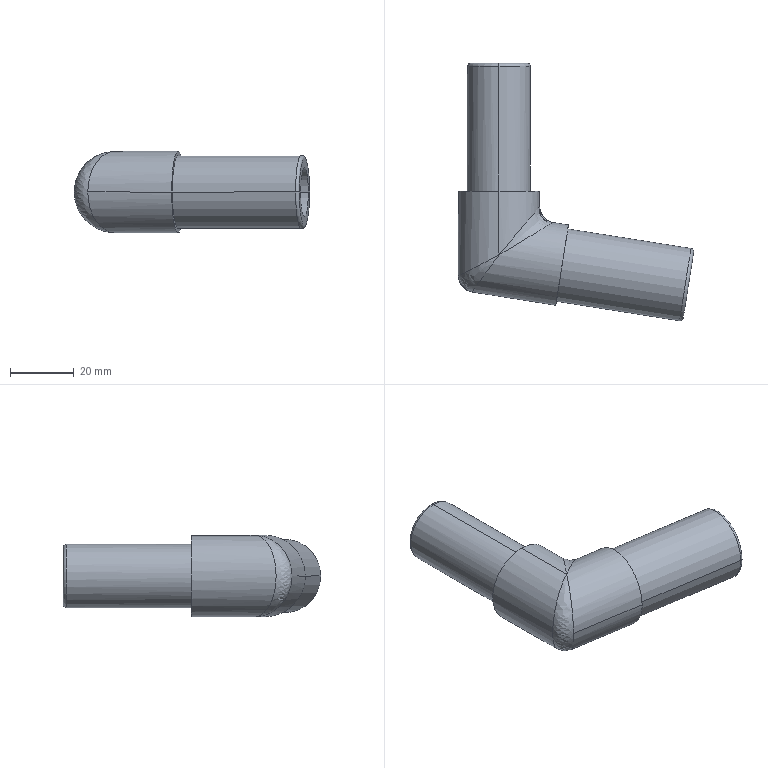Part | STEP file | 101000007608 | 1 solid | 25 faces | box 73.608 x 80.551 x 25.4 mm | volume 31663 mm3 | cylinder 14 | plane 5 | torus 4 | spline 2 | commonest cylinder face diameters 12.5 x4 25.4 x4 15.5 x2 19.8 x2 22.9 x2
STEP:
#1=CARTESIAN_POINT('',(-1.446,-20.539,0.));
#2=VERTEX_POINT('',#1);
#3=CARTESIAN_POINT('',(2.136,2.079,0.));
#4=VERTEX_POINT('',#3);
#5=CARTESIAN_POINT('',(0.345,-9.23,0.));
#6=DIRECTION('',(0.9877,-0.1564,0.));
#7=AXIS2_PLACEMENT_3D('',#5,#6,$);
#8=CIRCLE('',#7,11.45);
#9=EDGE_CURVE('',#2,#4,#8,.F.);
#10=ORIENTED_EDGE('',*,*,#9,.F.);
#11=CARTESIAN_POINT('',(-0.302,-19.707,0.));
#12=VERTEX_POINT('',#11);
#13=CARTESIAN_POINT('',(-1.29,-19.551,0.));
#14=DIRECTION('',(0.,0.,1.));
#15=AXIS2_PLACEMENT_3D('',#13,#14,$);
#16=CIRCLE('',#15,1.);
#17=EDGE_CURVE('',#2,#12,#16,.T.);
#18=ORIENTED_EDGE('',*,*,#17,.T.);
#19=CARTESIAN_POINT('',(2.967,0.9353,0.));
#20=VERTEX_POINT('',#19);
#21=CARTESIAN_POINT('',(1.333,-9.386,0.));
#22=DIRECTION('',(0.9877,-0.1564,0.));
#23=AXIS2_PLACEMENT_3D('',#21,#22,$);
#24=CIRCLE('',#23,10.45);
#25=EDGE_CURVE('',#20,#12,#24,.T.);
#26=ORIENTED_EDGE('',*,*,#25,.F.);
#27=CARTESIAN_POINT('',(1.98,1.092,0.));
#28=DIRECTION('',(0.,0.,-1.));
#29=AXIS2_PLACEMENT_3D('',#27,#28,$);
#30=CIRCLE('',#29,1.);
#31=EDGE_CURVE('',#4,#20,#30,.T.);
#32=ORIENTED_EDGE('',*,*,#31,.F.);
#33=EDGE_LOOP('',(#10,#18,#26,#32));
#34=FACE_OUTER_BOUND('',#33,.T.);
#35=CARTESIAN_POINT('',(0.345,-9.23,0.));
#36=DIRECTION('',(0.9877,-0.1564,0.));
#37=DIRECTION('',(0.1564,0.9877,0.));
#38=AXIS2_PLACEMENT_3D('',#35,#36,#37);
#39=TOROIDAL_SURFACE('',#38,10.45,1.);
#40=ADVANCED_FACE('',(#34),#39,.T.);
#41=ORIENTED_EDGE('',*,*,#9,.T.);
#42=CARTESIAN_POINT('',(-36.384,8.18,0.));
#43=VERTEX_POINT('',#42);
#44=CARTESIAN_POINT('',(3.124,1.923,0.));
#45=DIRECTION('',(-0.9877,0.1564,0.));
#46=VECTOR('',#45,1.);
#47=LINE('',#44,#46);
#48=EDGE_CURVE('',#4,#43,#47,.T.);
#49=ORIENTED_EDGE('',*,*,#48,.T.);
#50=CARTESIAN_POINT('',(-39.966,-14.438,0.));
#51=VERTEX_POINT('',#50);
#52=CARTESIAN_POINT('',(-38.175,-3.129,0.));
#53=DIRECTION('',(-0.9877,0.1564,0.));
#54=AXIS2_PLACEMENT_3D('',#52,#53,$);
#55=CIRCLE('',#54,11.45);
#56=EDGE_CURVE('',#43,#51,#55,.F.);
#57=ORIENTED_EDGE('',*,*,#56,.T.);
#58=CARTESIAN_POINT('',(-0.4585,-20.695,0.));
#59=DIRECTION('',(-0.9877,0.1564,0.));
#60=VECTOR('',#59,1.);
#61=LINE('',#58,#60);
#62=EDGE_CURVE('',#2,#51,#61,.T.);
#63=ORIENTED_EDGE('',*,*,#62,.F.);
#64=EDGE_LOOP('',(#41,#49,#57,#63));
#65=FACE_OUTER_BOUND('',#64,.T.);
#66=CARTESIAN_POINT('',(1.333,-9.386,0.));
#67=DIRECTION('',(-0.9877,0.1564,0.));
#68=DIRECTION('',(-0.1564,-0.9877,0.));
#69=AXIS2_PLACEMENT_3D('',#66,#67,#68);
#70=CYLINDRICAL_SURFACE('',#69,11.45);
#71=ADVANCED_FACE('',(#65),#70,.T.);
#72=ORIENTED_EDGE('',*,*,#17,.F.);
#73=CARTESIAN_POINT('',(0.345,-9.23,0.));
#74=DIRECTION('',(0.9877,-0.1564,0.));
#75=AXIS2_PLACEMENT_3D('',#73,#74,$);
#76=CIRCLE('',#75,11.45);
#77=EDGE_CURVE('',#4,#2,#76,.F.);
#78=ORIENTED_EDGE('',*,*,#77,.F.);
#79=ORIENTED_EDGE('',*,*,#31,.T.);
#80=CARTESIAN_POINT('',(1.333,-9.386,0.));
#81=DIRECTION('',(0.9877,-0.1564,0.));
#82=AXIS2_PLACEMENT_3D('',#80,#81,$);
#83=CIRCLE('',#82,10.45);
#84=EDGE_CURVE('',#12,#20,#83,.T.);
#85=ORIENTED_EDGE('',*,*,#84,.F.);
#86=EDGE_LOOP('',(#72,#78,#79,#85));
#87=FACE_OUTER_BOUND('',#86,.T.);
#88=CARTESIAN_POINT('',(0.345,-9.23,0.));
#89=DIRECTION('',(0.9877,-0.1564,0.));
#90=DIRECTION('',(-0.1564,-0.9877,0.));
#91=AXIS2_PLACEMENT_3D('',#88,#89,#90);
#92=TOROIDAL_SURFACE('',#91,10.45,1.);
#93=ADVANCED_FACE('',(#87),#92,.T.);
#94=ORIENTED_EDGE('',*,*,#25,.T.);
#95=ORIENTED_EDGE('',*,*,#84,.T.);
#96=EDGE_LOOP('',(#94,#95));
#97=FACE_OUTER_BOUND('',#96,.T.);
#98=CARTESIAN_POINT('',(2.545,-1.731,0.));
#99=VERTEX_POINT('',#98);
#100=CARTESIAN_POINT('',(0.1204,-17.041,0.));
#101=VERTEX_POINT('',#100);
#102=CARTESIAN_POINT('',(1.333,-9.386,0.));
#103=DIRECTION('',(0.9877,-0.1564,0.));
#104=AXIS2_PLACEMENT_3D('',#102,#103,$);
#105=CIRCLE('',#104,7.75);
#106=EDGE_CURVE('',#99,#101,#105,.T.);
#107=ORIENTED_EDGE('',*,*,#106,.F.);
#108=CARTESIAN_POINT('',(1.333,-9.386,0.));
#109=DIRECTION('',(0.9877,-0.1564,0.));
#110=AXIS2_PLACEMENT_3D('',#108,#109,$);
#111=CIRCLE('',#110,7.75);
#112=EDGE_CURVE('',#101,#99,#111,.T.);
#113=ORIENTED_EDGE('',*,*,#112,.F.);
#114=EDGE_LOOP('',(#107,#113));
#115=FACE_BOUND('',#114,.T.);
#116=CARTESIAN_POINT('',(1.333,-9.386,0.));
#117=DIRECTION('',(0.9877,-0.1564,0.));
#118=DIRECTION('',(0.1564,0.9877,0.));
#119=AXIS2_PLACEMENT_3D('',#116,#117,#118);
#120=PLANE('',#119);
#121=ADVANCED_FACE('',(#97,#115),#120,.T.);
#122=ORIENTED_EDGE('',*,*,#48,.F.);
#123=ORIENTED_EDGE('',*,*,#77,.T.);
#124=ORIENTED_EDGE('',*,*,#62,.T.);
#125=CARTESIAN_POINT('',(-38.175,-3.129,0.));
#126=DIRECTION('',(-0.9877,0.1564,0.));
#127=AXIS2_PLACEMENT_3D('',#125,#126,$);
#128=CIRCLE('',#127,11.45);
#129=EDGE_CURVE('',#51,#43,#128,.F.);
#130=ORIENTED_EDGE('',*,*,#129,.T.);
#131=EDGE_LOOP('',(#122,#123,#124,#130));
#132=FACE_OUTER_BOUND('',#131,.T.);
#133=CARTESIAN_POINT('',(1.333,-9.386,0.));
#134=DIRECTION('',(-0.9877,0.1564,0.));
#135=DIRECTION('',(0.1564,0.9877,0.));
#136=AXIS2_PLACEMENT_3D('',#133,#134,#135);
#137=CYLINDRICAL_SURFACE('',#136,11.45);
#138=ADVANCED_FACE('',(#132),#137,.T.);
#139=CARTESIAN_POINT('',(-36.188,9.415,0.));
#140=VERTEX_POINT('',#139);
#141=CARTESIAN_POINT('',(-40.162,-15.672,0.));
#142=VERTEX_POINT('',#141);
#143=CARTESIAN_POINT('',(-36.188,9.415,0.));
#144=CARTESIAN_POINT('',(-36.188,9.415,-1.222));
#145=CARTESIAN_POINT('',(-36.211,9.27,-2.444));
#146=CARTESIAN_POINT('',(-36.257,8.979,-3.643));
#147=CARTESIAN_POINT('',(-36.393,8.12,-5.945));
#148=CARTESIAN_POINT('',(-36.611,6.745,-7.976));
#149=CARTESIAN_POINT('',(-36.739,5.94,-8.902));
#150=CARTESIAN_POINT('',(-37.026,4.125,-10.541));
#151=CARTESIAN_POINT('',(-37.366,1.978,-11.697));
#152=CARTESIAN_POINT('',(-37.546,0.8408,-12.141));
#153=CARTESIAN_POINT('',(-37.92,-1.517,-12.743));
#154=CARTESIAN_POINT('',(-38.305,-3.948,-12.762));
#155=CARTESIAN_POINT('',(-38.496,-5.159,-12.622));
#156=CARTESIAN_POINT('',(-38.871,-7.525,-12.051));
#157=CARTESIAN_POINT('',(-39.214,-9.688,-10.929));
#158=CARTESIAN_POINT('',(-39.374,-10.698,-10.238));
#159=CARTESIAN_POINT('',(-39.664,-12.534,-8.624));
#160=CARTESIAN_POINT('',(-39.887,-13.939,-6.614));
#161=CARTESIAN_POINT('',(-39.979,-14.519,-5.529));
#162=CARTESIAN_POINT('',(-40.087,-15.199,-3.777));
#163=CARTESIAN_POINT('',(-40.142,-15.55,-1.938));
#164=CARTESIAN_POINT('',(-40.155,-15.632,-1.294));
#165=CARTESIAN_POINT('',(-40.162,-15.672,-0.6471));
#166=CARTESIAN_POINT('',(-40.162,-15.672,0.));
#167=B_SPLINE_CURVE_WITH_KNOTS('',5,(#143,#144,#145,#146,#147,#148,#149,#150,#151,#152,#153,#154,#155,#156,#157,#158,#159,#160,#161,#162,#163,#164,#165,#166),.UNSPECIFIED.,.F.,.U.,(6,3,3,3,3,3,3,6),(0.,8.641,17.283,25.924,34.566,43.207,51.849,56.424),.UNSPECIFIED.);
#168=EDGE_CURVE('',#140,#142,#167,.T.);
#169=ORIENTED_EDGE('',*,*,#168,.F.);
#170=CARTESIAN_POINT('',(-40.162,-15.672,0.));
#171=CARTESIAN_POINT('',(-40.162,-15.672,1.222));
#172=CARTESIAN_POINT('',(-40.139,-15.527,2.444));
#173=CARTESIAN_POINT('',(-40.093,-15.237,3.643));
#174=CARTESIAN_POINT('',(-39.956,-14.377,5.945));
#175=CARTESIAN_POINT('',(-39.739,-13.002,7.976));
#176=CARTESIAN_POINT('',(-39.611,-12.197,8.902));
#177=CARTESIAN_POINT('',(-39.324,-10.382,10.541));
#178=CARTESIAN_POINT('',(-38.984,-8.236,11.697));
#179=CARTESIAN_POINT('',(-38.804,-7.098,12.141));
#180=CARTESIAN_POINT('',(-38.43,-4.741,12.743));
#181=CARTESIAN_POINT('',(-38.045,-2.309,12.762));
#182=CARTESIAN_POINT('',(-37.853,-1.098,12.622));
#183=CARTESIAN_POINT('',(-37.479,1.267,12.051));
#184=CARTESIAN_POINT('',(-37.136,3.431,10.929));
#185=CARTESIAN_POINT('',(-36.976,4.441,10.238));
#186=CARTESIAN_POINT('',(-36.685,6.277,8.624));
#187=CARTESIAN_POINT('',(-36.463,7.682,6.614));
#188=CARTESIAN_POINT('',(-36.371,8.261,5.529));
#189=CARTESIAN_POINT('',(-36.263,8.941,3.777));
#190=CARTESIAN_POINT('',(-36.207,9.293,1.938));
#191=CARTESIAN_POINT('',(-36.195,9.374,1.294));
#192=CARTESIAN_POINT('',(-36.188,9.415,0.6471));
#193=CARTESIAN_POINT('',(-36.188,9.415,0.));
#194=B_SPLINE_CURVE_WITH_KNOTS('',5,(#170,#171,#172,#173,#174,#175,#176,#177,#178,#179,#180,#181,#182,#183,#184,#185,#186,#187,#188,#189,#190,#191,#192,#193),.UNSPECIFIED.,.F.,.U.,(6,3,3,3,3,3,3,6),(0.,8.641,17.283,25.924,34.566,43.207,51.849,56.424),.UNSPECIFIED.);
#195=EDGE_CURVE('',#142,#140,#194,.T.);
#196=ORIENTED_EDGE('',*,*,#195,.F.);
#197=EDGE_LOOP('',(#169,#196));
#198=FACE_OUTER_BOUND('',#197,.T.);
#199=ORIENTED_EDGE('',*,*,#129,.F.);
#200=ORIENTED_EDGE('',*,*,#56,.F.);
#201=EDGE_LOOP('',(#199,#200));
#202=FACE_BOUND('',#201,.T.);
#203=CARTESIAN_POINT('',(-38.175,-3.129,0.));
#204=DIRECTION('',(0.9877,-0.1564,0.));
#205=DIRECTION('',(0.1564,0.9877,0.));
#206=AXIS2_PLACEMENT_3D('',#203,#204,#205);
#207=PLANE('',#206);
#208=ADVANCED_FACE('',(#198,#202),#207,.T.);
#209=CARTESIAN_POINT('',(-39.387,-10.783,0.));
#210=VERTEX_POINT('',#209);
#211=CARTESIAN_POINT('',(-61.038,-7.354,0.));
#212=DIRECTION('',(0.9877,-0.1564,0.));
#213=VECTOR('',#212,1.);
#214=LINE('',#211,#213);
#215=EDGE_CURVE('',#210,#101,#214,.T.);
#216=ORIENTED_EDGE('',*,*,#215,.F.);
#217=CARTESIAN_POINT('',(-36.962,4.526,0.));
#218=VERTEX_POINT('',#217);
#219=CARTESIAN_POINT('',(-38.175,-3.129,0.));
#220=DIRECTION('',(0.9877,-0.1564,0.));
#221=AXIS2_PLACEMENT_3D('',#219,#220,$);
#222=CIRCLE('',#221,7.75);
#223=EDGE_CURVE('',#210,#218,#222,.F.);
#224=ORIENTED_EDGE('',*,*,#223,.T.);
#225=CARTESIAN_POINT('',(-58.613,7.955,0.));
#226=DIRECTION('',(0.9877,-0.1564,0.));
#227=VECTOR('',#226,1.);
#228=LINE('',#225,#227);
#229=EDGE_CURVE('',#218,#99,#228,.T.);
#230=ORIENTED_EDGE('',*,*,#229,.T.);
#231=ORIENTED_EDGE('',*,*,#106,.T.);
#232=EDGE_LOOP('',(#216,#224,#230,#231));
#233=FACE_OUTER_BOUND('',#232,.T.);
#234=CARTESIAN_POINT('',(-59.825,0.3004,0.));
#235=DIRECTION('',(0.9877,-0.1564,0.));
#236=DIRECTION('',(0.1564,0.9877,0.));
#237=AXIS2_PLACEMENT_3D('',#234,#235,#236);
#238=CYLINDRICAL_SURFACE('',#237,7.75);
#239=ADVANCED_FACE('',(#233),#238,.F.);
#240=CARTESIAN_POINT('',(-38.175,-3.129,0.));
#241=DIRECTION('',(0.9877,-0.1564,0.));
#242=AXIS2_PLACEMENT_3D('',#240,#241,$);
#243=CIRCLE('',#242,7.75);
#244=EDGE_CURVE('',#218,#210,#243,.F.);
#245=ORIENTED_EDGE('',*,*,#244,.T.);
#246=ORIENTED_EDGE('',*,*,#215,.T.);
#247=ORIENTED_EDGE('',*,*,#112,.T.);
#248=ORIENTED_EDGE('',*,*,#229,.F.);
#249=EDGE_LOOP('',(#245,#246,#247,#248));
#250=FACE_OUTER_BOUND('',#249,.T.);
#251=CARTESIAN_POINT('',(-59.825,0.3004,0.));
#252=DIRECTION('',(0.9877,-0.1564,0.));
#253=DIRECTION('',(-0.1564,-0.9877,0.));
#254=AXIS2_PLACEMENT_3D('',#251,#252,#253);
#255=CYLINDRICAL_SURFACE('',#254,7.75);
#256=ADVANCED_FACE('',(#250),#255,.F.);
#257=CARTESIAN_POINT('',(-66.411,-11.515,0.));
#258=VERTEX_POINT('',#257);
#259=CARTESIAN_POINT('',(-59.915,-12.544,0.));
#260=DIRECTION('',(0.9877,-0.1564,0.));
#261=VECTOR('',#260,1.);
#262=LINE('',#259,#261);
#263=EDGE_CURVE('',#258,#142,#262,.T.);
#264=ORIENTED_EDGE('',*,*,#263,.F.);
#265=CARTESIAN_POINT('',(-57.929,0.,-12.7));
#266=VERTEX_POINT('',#265);
#267=CARTESIAN_POINT('',(-66.411,-11.515,0.));
#268=CARTESIAN_POINT('',(-66.411,-11.515,-1.568));
#269=CARTESIAN_POINT('',(-66.249,-11.295,-3.2));
#270=CARTESIAN_POINT('',(-65.899,-10.82,-4.82));
#271=CARTESIAN_POINT('',(-64.754,-9.265,-8.073));
#272=CARTESIAN_POINT('',(-62.932,-6.792,-10.53));
#273=CARTESIAN_POINT('',(-61.813,-5.274,-11.523));
#274=CARTESIAN_POINT('',(-60.329,-3.258,-12.336));
#275=CARTESIAN_POINT('',(-58.845,-1.245,-12.638));
#276=CARTESIAN_POINT('',(-58.537,-0.8263,-12.68));
#277=CARTESIAN_POINT('',(-58.231,-0.4109,-12.7));
#278=CARTESIAN_POINT('',(-57.929,0.,-12.7));
#279=B_SPLINE_CURVE_WITH_KNOTS('',5,(#267,#268,#269,#270,#271,#272,#273,#274,#275,#276,#277,#278),.UNSPECIFIED.,.F.,.U.,(6,3,3,6),(0.,12.994,27.923,31.858),.UNSPECIFIED.);
#280=EDGE_CURVE('',#258,#266,#279,.T.);
#281=ORIENTED_EDGE('',*,*,#280,.T.);
#282=CARTESIAN_POINT('',(-41.011,10.179,0.));
#283=VERTEX_POINT('',#282);
#284=CARTESIAN_POINT('',(-57.929,0.,-12.7));
#285=CARTESIAN_POINT('',(-55.645,1.374,-12.7));
#286=CARTESIAN_POINT('',(-53.28,2.797,-12.411));
#287=CARTESIAN_POINT('',(-50.904,4.226,-11.789));
#288=CARTESIAN_POINT('',(-47.169,6.474,-10.16));
#289=CARTESIAN_POINT('',(-44.169,8.279,-7.576));
#290=CARTESIAN_POINT('',(-43.138,8.899,-6.405));
#291=CARTESIAN_POINT('',(-41.886,9.652,-4.402));
#292=CARTESIAN_POINT('',(-41.236,10.043,-2.276));
#293=CARTESIAN_POINT('',(-41.084,10.135,-1.508));
#294=CARTESIAN_POINT('',(-41.011,10.179,-0.7456));
#295=CARTESIAN_POINT('',(-41.011,10.179,0.));
#296=B_SPLINE_CURVE_WITH_KNOTS('',5,(#284,#285,#286,#287,#288,#289,#290,#291,#292,#293,#294,#295),.UNSPECIFIED.,.F.,.U.,(6,3,3,6),(0.,19.117,31.662,38.695),.UNSPECIFIED.);
#297=EDGE_CURVE('',#266,#283,#296,.T.);
#298=ORIENTED_EDGE('',*,*,#297,.T.);
#299=CARTESIAN_POINT('',(-55.942,12.544,0.));
#300=DIRECTION('',(0.9877,-0.1564,0.));
#301=VECTOR('',#300,1.);
#302=LINE('',#299,#301);
#303=EDGE_CURVE('',#283,#140,#302,.T.);
#304=ORIENTED_EDGE('',*,*,#303,.T.);
#305=ORIENTED_EDGE('',*,*,#168,.T.);
#306=EDGE_LOOP('',(#264,#281,#298,#304,#305));
#307=FACE_OUTER_BOUND('',#306,.T.);
#308=CARTESIAN_POINT('',(-57.929,0.,0.));
#309=DIRECTION('',(0.9877,-0.1564,0.));
#310=DIRECTION('',(-0.1564,-0.9877,0.));
#311=AXIS2_PLACEMENT_3D('',#308,#309,#310);
#312=CYLINDRICAL_SURFACE('',#311,12.7);
#313=ADVANCED_FACE('',(#307),#312,.T.);
#314=CARTESIAN_POINT('',(-57.929,0.,12.7));
#315=VERTEX_POINT('',#314);
#316=CARTESIAN_POINT('',(-57.929,0.,12.7));
#317=CARTESIAN_POINT('',(-59.109,-1.603,12.7));
#318=CARTESIAN_POINT('',(-60.339,-3.272,12.392));
#319=CARTESIAN_POINT('',(-61.565,-4.936,11.723));
#320=CARTESIAN_POINT('',(-63.651,-7.769,9.814));
#321=CARTESIAN_POINT('',(-65.191,-9.859,6.885));
#322=CARTESIAN_POINT('',(-65.738,-10.602,5.373));
#323=CARTESIAN_POINT('',(-66.199,-11.227,3.336));
#324=CARTESIAN_POINT('',(-66.374,-11.465,1.298));
#325=CARTESIAN_POINT('',(-66.399,-11.498,0.8615));
#326=CARTESIAN_POINT('',(-66.411,-11.515,0.4284));
#327=CARTESIAN_POINT('',(-66.411,-11.515,0.));
#328=B_SPLINE_CURVE_WITH_KNOTS('',5,(#316,#317,#318,#319,#320,#321,#322,#323,#324,#325,#326,#327),.UNSPECIFIED.,.F.,.U.,(6,3,3,6),(0.,15.347,28.306,31.856),.UNSPECIFIED.);
#329=EDGE_CURVE('',#315,#258,#328,.T.);
#330=ORIENTED_EDGE('',*,*,#329,.T.);
#331=ORIENTED_EDGE('',*,*,#263,.T.);
#332=ORIENTED_EDGE('',*,*,#195,.T.);
#333=ORIENTED_EDGE('',*,*,#303,.F.);
#334=CARTESIAN_POINT('',(-41.011,10.179,0.));
#335=CARTESIAN_POINT('',(-41.011,10.179,1.241));
#336=CARTESIAN_POINT('',(-41.213,10.057,2.527));
#337=CARTESIAN_POINT('',(-41.646,9.796,3.81));
#338=CARTESIAN_POINT('',(-43.061,8.945,6.454));
#339=CARTESIAN_POINT('',(-45.318,7.587,8.658));
#340=CARTESIAN_POINT('',(-46.72,6.744,9.667));
#341=CARTESIAN_POINT('',(-49.725,4.935,11.31));
#342=CARTESIAN_POINT('',(-53.007,2.961,12.254));
#343=CARTESIAN_POINT('',(-54.668,1.962,12.556));
#344=CARTESIAN_POINT('',(-56.319,0.9686,12.7));
#345=CARTESIAN_POINT('',(-57.929,0.,12.7));
#346=B_SPLINE_CURVE_WITH_KNOTS('',5,(#334,#335,#336,#337,#338,#339,#340,#341,#342,#343,#344,#345),.UNSPECIFIED.,.F.,.U.,(6,3,3,6),(0.,11.707,25.241,38.719),.UNSPECIFIED.);
#347=EDGE_CURVE('',#283,#315,#346,.T.);
#348=ORIENTED_EDGE('',*,*,#347,.T.);
#349=EDGE_LOOP('',(#330,#331,#332,#333,#348));
#350=FACE_OUTER_BOUND('',#349,.T.);
#351=CARTESIAN_POINT('',(-57.929,0.,0.));
#352=DIRECTION('',(0.9877,-0.1564,0.));
#353=DIRECTION('',(0.1564,0.9877,0.));
#354=AXIS2_PLACEMENT_3D('',#351,#352,#353);
#355=CYLINDRICAL_SURFACE('',#354,12.7);
#356=ADVANCED_FACE('',(#350),#355,.T.);
#357=ORIENTED_EDGE('',*,*,#244,.F.);
#358=ORIENTED_EDGE('',*,*,#223,.F.);
#359=EDGE_LOOP('',(#357,#358));
#360=FACE_OUTER_BOUND('',#359,.T.);
#361=CARTESIAN_POINT('',(-37.197,3.044,0.));
#362=VERTEX_POINT('',#361);
#363=CARTESIAN_POINT('',(-39.153,-9.302,0.));
#364=VERTEX_POINT('',#363);
#365=CARTESIAN_POINT('',(-37.197,3.044,0.));
#366=CARTESIAN_POINT('',(-37.197,3.044,-0.6124));
#367=CARTESIAN_POINT('',(-37.209,2.97,-1.225));
#368=CARTESIAN_POINT('',(-37.232,2.822,-1.825));
#369=CARTESIAN_POINT('',(-37.302,2.384,-2.976));
#370=CARTESIAN_POINT('',(-37.413,1.684,-3.986));
#371=CARTESIAN_POINT('',(-37.477,1.274,-4.445));
#372=CARTESIAN_POINT('',(-37.624,0.3522,-5.252));
#373=CARTESIAN_POINT('',(-37.796,-0.7349,-5.81));
#374=CARTESIAN_POINT('',(-37.887,-1.31,-6.02));
#375=CARTESIAN_POINT('',(-38.075,-2.498,-6.293));
#376=CARTESIAN_POINT('',(-38.268,-3.717,-6.267));
#377=CARTESIAN_POINT('',(-38.364,-4.321,-6.178));
#378=CARTESIAN_POINT('',(-38.55,-5.497,-5.853));
#379=CARTESIAN_POINT('',(-38.718,-6.56,-5.25));
#380=CARTESIAN_POINT('',(-38.796,-7.052,-4.884));
#381=CARTESIAN_POINT('',(-38.937,-7.938,-4.036));
#382=CARTESIAN_POINT('',(-39.041,-8.596,-2.998));
#383=CARTESIAN_POINT('',(-39.083,-8.86,-2.44));
#384=CARTESIAN_POINT('',(-39.126,-9.135,-1.614));
#385=CARTESIAN_POINT('',(-39.147,-9.264,-0.7578));
#386=CARTESIAN_POINT('',(-39.151,-9.289,-0.5051));
#387=CARTESIAN_POINT('',(-39.153,-9.302,-0.2525));
#388=CARTESIAN_POINT('',(-39.153,-9.302,0.));
#389=B_SPLINE_CURVE_WITH_KNOTS('',5,(#365,#366,#367,#368,#369,#370,#371,#372,#373,#374,#375,#376,#377,#378,#379,#380,#381,#382,#383,#384,#385,#386,#387,#388),.UNSPECIFIED.,.F.,.U.,(6,3,3,3,3,3,3,6),(0.,4.33,8.66,12.99,17.32,21.65,25.98,27.766),.UNSPECIFIED.);
#390=EDGE_CURVE('',#362,#364,#389,.T.);
#391=ORIENTED_EDGE('',*,*,#390,.T.);
#392=CARTESIAN_POINT('',(-39.153,-9.302,0.));
#393=CARTESIAN_POINT('',(-39.153,-9.302,0.6124));
#394=CARTESIAN_POINT('',(-39.141,-9.228,1.225));
#395=CARTESIAN_POINT('',(-39.117,-9.079,1.825));
#396=CARTESIAN_POINT('',(-39.048,-8.641,2.976));
#397=CARTESIAN_POINT('',(-38.937,-7.941,3.986));
#398=CARTESIAN_POINT('',(-38.872,-7.531,4.445));
#399=CARTESIAN_POINT('',(-38.726,-6.61,5.252));
#400=CARTESIAN_POINT('',(-38.554,-5.523,5.81));
#401=CARTESIAN_POINT('',(-38.463,-4.948,6.02));
#402=CARTESIAN_POINT('',(-38.275,-3.759,6.293));
#403=CARTESIAN_POINT('',(-38.082,-2.541,6.267));
#404=CARTESIAN_POINT('',(-37.986,-1.936,6.178));
#405=CARTESIAN_POINT('',(-37.8,-0.7606,5.853));
#406=CARTESIAN_POINT('',(-37.631,0.3026,5.25));
#407=CARTESIAN_POINT('',(-37.553,0.795,4.884));
#408=CARTESIAN_POINT('',(-37.413,1.681,4.036));
#409=CARTESIAN_POINT('',(-37.309,2.339,2.998));
#410=CARTESIAN_POINT('',(-37.267,2.603,2.44));
#411=CARTESIAN_POINT('',(-37.224,2.877,1.614));
#412=CARTESIAN_POINT('',(-37.203,3.006,0.7578));
#413=CARTESIAN_POINT('',(-37.199,3.032,0.5051));
#414=CARTESIAN_POINT('',(-37.197,3.044,0.2525));
#415=CARTESIAN_POINT('',(-37.197,3.044,0.));
#416=B_SPLINE_CURVE_WITH_KNOTS('',5,(#392,#393,#394,#395,#396,#397,#398,#399,#400,#401,#402,#403,#404,#405,#406,#407,#408,#409,#410,#411,#412,#413,#414,#415),.UNSPECIFIED.,.F.,.U.,(6,3,3,3,3,3,3,6),(0.,4.33,8.66,12.99,17.32,21.65,25.98,27.766),.UNSPECIFIED.);
#417=EDGE_CURVE('',#364,#362,#416,.T.);
#418=ORIENTED_EDGE('',*,*,#417,.T.);
#419=EDGE_LOOP('',(#391,#418));
#420=FACE_BOUND('',#419,.T.);
#421=CARTESIAN_POINT('',(-38.175,-3.129,0.));
#422=DIRECTION('',(0.9877,-0.1564,0.));
#423=DIRECTION('',(0.1564,0.9877,0.));
#424=AXIS2_PLACEMENT_3D('',#421,#422,#423);
#425=PLANE('',#424);
#426=ADVANCED_FACE('',(#360,#420),#425,.T.);
#427=ORIENTED_EDGE('',*,*,#329,.F.);
#428=CARTESIAN_POINT('',(-57.929,0.,12.7));
#429=CARTESIAN_POINT('',(-59.592,-0.8611,12.701));
#430=CARTESIAN_POINT('',(-62.083,-2.151,12.203));
#431=CARTESIAN_POINT('',(-65.767,-4.059,10.235));
#432=CARTESIAN_POINT('',(-68.164,-5.3,7.839));
#433=CARTESIAN_POINT('',(-69.737,-6.115,4.891));
#434=CARTESIAN_POINT('',(-70.465,-6.492,2.494));
#435=CARTESIAN_POINT('',(-70.71,-6.619,0.));
#436=CARTESIAN_POINT('',(-70.465,-6.492,-2.494));
#437=CARTESIAN_POINT('',(-69.737,-6.115,-4.891));
#438=CARTESIAN_POINT('',(-68.164,-5.3,-7.839));
#439=CARTESIAN_POINT('',(-65.767,-4.059,-10.235));
#440=CARTESIAN_POINT('',(-62.083,-2.151,-12.203));
#441=CARTESIAN_POINT('',(-59.592,-0.8611,-12.701));
#442=CARTESIAN_POINT('',(-57.929,0.,-12.7));
#443=(BOUNDED_CURVE()B_SPLINE_CURVE(3,(#428,#429,#430,#431,#432,#433,#434,#435,#436,#437,#438,#439,#440,#441,#442),.UNSPECIFIED.,.F.,.U.)B_SPLINE_CURVE_WITH_KNOTS((4,1,1,1,1,1,1,1,1,1,1,1,4),(1.571,7.061,9.806,15.296,18.041,20.787,23.532,26.277,29.022,31.767,37.257,40.002,45.492),.UNSPECIFIED.)CURVE()GEOMETRIC_REPRESENTATION_ITEM()RATIONAL_B_SPLINE_CURVE((1.,1.,1.,1.,1.,1.,1.,1.,1.,1.,1.,1.,1.,1.,1.))REPRESENTATION_ITEM(''));
#444=EDGE_CURVE('',#266,#315,#443,.F.);
#445=ORIENTED_EDGE('',*,*,#444,.F.);
#446=ORIENTED_EDGE('',*,*,#280,.F.);
#447=EDGE_LOOP('',(#427,#445,#446));
#448=FACE_OUTER_BOUND('',#447,.T.);
#449=CARTESIAN_POINT('',(-57.929,0.,12.7));
#450=CARTESIAN_POINT('',(-57.929,0.,12.7));
#451=CARTESIAN_POINT('',(-57.929,0.,12.7));
#452=CARTESIAN_POINT('',(-59.592,-0.8611,12.701));
#453=CARTESIAN_POINT('',(-59.315,-1.184,12.7));
#454=CARTESIAN_POINT('',(-59.039,-1.508,12.701));
#455=CARTESIAN_POINT('',(-62.083,-2.151,12.203));
#456=CARTESIAN_POINT('',(-61.447,-3.005,12.363));
#457=CARTESIAN_POINT('',(-60.703,-3.767,12.203));
#458=CARTESIAN_POINT('',(-65.767,-4.059,10.235));
#459=CARTESIAN_POINT('',(-64.804,-5.872,10.929));
#460=CARTESIAN_POINT('',(-63.164,-7.107,10.235));
#461=CARTESIAN_POINT('',(-68.164,-5.3,7.839));
#462=CARTESIAN_POINT('',(-67.329,-8.028,8.955));
#463=CARTESIAN_POINT('',(-64.765,-9.28,7.839));
#464=CARTESIAN_POINT('',(-69.737,-6.115,4.891));
#465=CARTESIAN_POINT('',(-69.311,-9.722,5.99));
#466=CARTESIAN_POINT('',(-65.815,-10.707,4.891));
#467=CARTESIAN_POINT('',(-70.465,-6.492,2.494));
#468=CARTESIAN_POINT('',(-70.372,-10.627,3.179));
#469=CARTESIAN_POINT('',(-66.302,-11.367,2.494));
#470=CARTESIAN_POINT('',(-70.71,-6.619,0.));
#471=CARTESIAN_POINT('',(-70.759,-10.958,0.));
#472=CARTESIAN_POINT('',(-66.465,-11.589,0.));
#473=CARTESIAN_POINT('',(-70.465,-6.492,-2.494));
#474=CARTESIAN_POINT('',(-70.372,-10.627,-3.179));
#475=CARTESIAN_POINT('',(-66.302,-11.367,-2.494));
#476=CARTESIAN_POINT('',(-69.737,-6.115,-4.891));
#477=CARTESIAN_POINT('',(-69.311,-9.722,-5.99));
#478=CARTESIAN_POINT('',(-65.815,-10.707,-4.891));
#479=CARTESIAN_POINT('',(-68.164,-5.3,-7.839));
#480=CARTESIAN_POINT('',(-67.329,-8.028,-8.955));
#481=CARTESIAN_POINT('',(-64.765,-9.28,-7.839));
#482=CARTESIAN_POINT('',(-65.767,-4.059,-10.235));
#483=CARTESIAN_POINT('',(-64.804,-5.872,-10.929));
#484=CARTESIAN_POINT('',(-63.164,-7.107,-10.235));
#485=CARTESIAN_POINT('',(-62.083,-2.151,-12.203));
#486=CARTESIAN_POINT('',(-61.447,-3.005,-12.363));
#487=CARTESIAN_POINT('',(-60.703,-3.767,-12.203));
#488=CARTESIAN_POINT('',(-59.592,-0.8611,-12.701));
#489=CARTESIAN_POINT('',(-59.315,-1.184,-12.7));
#490=CARTESIAN_POINT('',(-59.039,-1.508,-12.701));
#491=CARTESIAN_POINT('',(-57.929,0.,-12.7));
#492=CARTESIAN_POINT('',(-57.929,0.,-12.7));
#493=CARTESIAN_POINT('',(-57.929,0.,-12.7));
#494=(BOUNDED_SURFACE()B_SPLINE_SURFACE(3,2,((#449,#450,#451),(#452,#453,#454),(#455,#456,#457),(#458,#459,#460),(#461,#462,#463),(#464,#465,#466),(#467,#468,#469),(#470,#471,#472),(#473,#474,#475),(#476,#477,#478),(#479,#480,#481),(#482,#483,#484),(#485,#486,#487),(#488,#489,#490),(#491,#492,#493)),.UNSPECIFIED.,.F.,.F.,.U.)B_SPLINE_SURFACE_WITH_KNOTS((4,1,1,1,1,1,1,1,1,1,1,1,4),(3,3),(1.571,7.061,9.806,15.296,18.041,20.787,23.532,26.277,29.022,31.767,37.257,40.002,45.492),(0.,5.11),.UNSPECIFIED.)GEOMETRIC_REPRESENTATION_ITEM()RATIONAL_B_SPLINE_SURFACE(((1.,1.,1.),(1.,1.,1.),(1.,0.983,1.),(1.,0.9219,1.),(1.,0.8553,1.),(1.,0.7978,1.),(1.,0.7677,1.),(1.,0.7568,1.),(1.,0.7677,1.),(1.,0.7978,1.),(1.,0.8553,1.),(1.,0.9219,1.),(1.,0.983,1.),(1.,1.,1.),(1.,1.,1.)))REPRESENTATION_ITEM('')SURFACE());
#495=ADVANCED_FACE('',(#448),#494,.T.);
#496=ORIENTED_EDGE('',*,*,#297,.F.);
#497=CARTESIAN_POINT('',(-57.929,0.,-12.7));
#498=CARTESIAN_POINT('',(-57.097,0.9894,-12.7));
#499=CARTESIAN_POINT('',(-55.435,2.968,-12.536));
#500=CARTESIAN_POINT('',(-53.037,5.822,-11.809));
#501=CARTESIAN_POINT('',(-50.827,8.453,-10.628));
#502=CARTESIAN_POINT('',(-48.89,10.758,-9.038));
#503=CARTESIAN_POINT('',(-47.301,12.651,-7.101));
#504=CARTESIAN_POINT('',(-46.12,14.057,-4.891));
#505=CARTESIAN_POINT('',(-45.392,14.922,-2.494));
#506=CARTESIAN_POINT('',(-45.147,15.215,0.));
#507=CARTESIAN_POINT('',(-45.392,14.922,2.494));
#508=CARTESIAN_POINT('',(-46.12,14.057,4.891));
#509=CARTESIAN_POINT('',(-47.301,12.651,7.101));
#510=CARTESIAN_POINT('',(-48.89,10.758,9.038));
#511=CARTESIAN_POINT('',(-50.827,8.453,10.628));
#512=CARTESIAN_POINT('',(-53.037,5.822,11.809));
#513=CARTESIAN_POINT('',(-55.435,2.968,12.536));
#514=CARTESIAN_POINT('',(-57.097,0.9894,12.7));
#515=CARTESIAN_POINT('',(-57.929,0.,12.7));
#516=(BOUNDED_CURVE()B_SPLINE_CURVE(3,(#497,#498,#499,#500,#501,#502,#503,#504,#505,#506,#507,#508,#509,#510,#511,#512,#513,#514,#515),.UNSPECIFIED.,.F.,.U.)B_SPLINE_CURVE_WITH_KNOTS((4,1,1,1,1,1,1,1,1,1,1,1,1,1,1,1,4),(4.712,7.836,10.959,14.082,17.205,20.329,23.452,26.575,29.698,32.822,35.945,39.068,42.191,45.315,48.438,51.561,54.684),.UNSPECIFIED.)CURVE()GEOMETRIC_REPRESENTATION_ITEM()RATIONAL_B_SPLINE_CURVE((1.,1.,1.,1.,1.,1.,1.,1.,1.,1.,1.,1.,1.,1.,1.,1.,1.,1.,1.))REPRESENTATION_ITEM(''));
#517=EDGE_CURVE('',#315,#266,#516,.F.);
#518=ORIENTED_EDGE('',*,*,#517,.F.);
#519=ORIENTED_EDGE('',*,*,#347,.F.);
#520=EDGE_LOOP('',(#496,#518,#519));
#521=FACE_OUTER_BOUND('',#520,.T.);
#522=CARTESIAN_POINT('',(-57.929,0.,-12.7));
#523=CARTESIAN_POINT('',(-57.929,0.,-12.7));
#524=CARTESIAN_POINT('',(-57.929,0.,-12.7));
#525=CARTESIAN_POINT('',(-56.821,0.6662,-12.7));
#526=CARTESIAN_POINT('',(-56.959,0.8278,-12.7));
#527=CARTESIAN_POINT('',(-57.097,0.9894,-12.7));
#528=CARTESIAN_POINT('',(-54.607,1.999,-12.536));
#529=CARTESIAN_POINT('',(-55.005,2.497,-12.478));
#530=CARTESIAN_POINT('',(-55.435,2.968,-12.536));
#531=CARTESIAN_POINT('',(-51.413,3.92,-11.809));
#532=CARTESIAN_POINT('',(-52.252,4.848,-11.509));
#533=CARTESIAN_POINT('',(-53.037,5.822,-11.809));
#534=CARTESIAN_POINT('',(-48.469,5.691,-10.628));
#535=CARTESIAN_POINT('',(-49.831,6.916,-9.981));
#536=CARTESIAN_POINT('',(-50.827,8.453,-10.628));
#537=CARTESIAN_POINT('',(-45.889,7.244,-9.038));
#538=CARTESIAN_POINT('',(-47.881,8.582,-8.036));
#539=CARTESIAN_POINT('',(-48.89,10.758,-9.038));
#540=CARTESIAN_POINT('',(-43.771,8.518,-7.101));
#541=CARTESIAN_POINT('',(-46.491,9.769,-5.871));
#542=CARTESIAN_POINT('',(-47.301,12.651,-7.101));
#543=CARTESIAN_POINT('',(-42.198,9.465,-4.891));
#544=CARTESIAN_POINT('',(-45.664,10.475,-3.72));
#545=CARTESIAN_POINT('',(-46.12,14.057,-4.891));
#546=CARTESIAN_POINT('',(-41.229,10.048,-2.494));
#547=CARTESIAN_POINT('',(-45.291,10.793,-1.762));
#548=CARTESIAN_POINT('',(-45.392,14.922,-2.494));
#549=CARTESIAN_POINT('',(-40.902,10.244,0.));
#550=CARTESIAN_POINT('',(-45.197,10.874,0.));
#551=CARTESIAN_POINT('',(-45.147,15.215,0.));
#552=CARTESIAN_POINT('',(-41.229,10.048,2.494));
#553=CARTESIAN_POINT('',(-45.291,10.793,1.762));
#554=CARTESIAN_POINT('',(-45.392,14.922,2.494));
#555=CARTESIAN_POINT('',(-42.198,9.465,4.891));
#556=CARTESIAN_POINT('',(-45.664,10.475,3.72));
#557=CARTESIAN_POINT('',(-46.12,14.057,4.891));
#558=CARTESIAN_POINT('',(-43.771,8.518,7.101));
#559=CARTESIAN_POINT('',(-46.491,9.769,5.871));
#560=CARTESIAN_POINT('',(-47.301,12.651,7.101));
#561=CARTESIAN_POINT('',(-45.889,7.244,9.038));
#562=CARTESIAN_POINT('',(-47.881,8.582,8.036));
#563=CARTESIAN_POINT('',(-48.89,10.758,9.038));
#564=CARTESIAN_POINT('',(-48.469,5.691,10.628));
#565=CARTESIAN_POINT('',(-49.831,6.916,9.981));
#566=CARTESIAN_POINT('',(-50.827,8.453,10.628));
#567=CARTESIAN_POINT('',(-51.413,3.92,11.809));
#568=CARTESIAN_POINT('',(-52.252,4.848,11.509));
#569=CARTESIAN_POINT('',(-53.037,5.822,11.809));
#570=CARTESIAN_POINT('',(-54.607,1.999,12.536));
#571=CARTESIAN_POINT('',(-55.005,2.497,12.478));
#572=CARTESIAN_POINT('',(-55.435,2.968,12.536));
#573=CARTESIAN_POINT('',(-56.821,0.6662,12.7));
#574=CARTESIAN_POINT('',(-56.959,0.8278,12.7));
#575=CARTESIAN_POINT('',(-57.097,0.9894,12.7));
#576=CARTESIAN_POINT('',(-57.929,0.,12.7));
#577=CARTESIAN_POINT('',(-57.929,0.,12.7));
#578=CARTESIAN_POINT('',(-57.929,0.,12.7));
#579=(BOUNDED_SURFACE()B_SPLINE_SURFACE(3,2,((#522,#523,#524),(#525,#526,#527),(#528,#529,#530),(#531,#532,#533),(#534,#535,#536),(#537,#538,#539),(#540,#541,#542),(#543,#544,#545),(#546,#547,#548),(#549,#550,#551),(#552,#553,#554),(#555,#556,#557),(#558,#559,#560),(#561,#562,#563),(#564,#565,#566),(#567,#568,#569),(#570,#571,#572),(#573,#574,#575),(#576,#577,#578)),.UNSPECIFIED.,.F.,.F.,.U.)B_SPLINE_SURFACE_WITH_KNOTS((4,1,1,1,1,1,1,1,1,1,1,1,1,1,1,1,4),(3,3),(4.712,7.836,10.959,14.082,17.205,20.329,23.452,26.575,29.698,32.822,35.945,39.068,42.191,45.315,48.438,51.561,54.684),(0.,4.659),.UNSPECIFIED.)GEOMETRIC_REPRESENTATION_ITEM()RATIONAL_B_SPLINE_SURFACE(((1.,1.,1.),(1.,1.,1.),(1.,0.9945,1.),(1.,0.9708,1.),(1.,0.9341,1.),(1.,0.8887,1.),(1.,0.8409,1.),(1.,0.7979,1.),(1.,0.7677,1.),(1.,0.7568,1.),(1.,0.7677,1.),(1.,0.7979,1.),(1.,0.8409,1.),(1.,0.8887,1.),(1.,0.9341,1.),(1.,0.9708,1.),(1.,0.9945,1.),(1.,1.,1.),(1.,1.,1.)))REPRESENTATION_ITEM('')SURFACE());
#580=ADVANCED_FACE('',(#521),#579,.F.);
#581=CARTESIAN_POINT('',(-64.179,-5.338,0.));
#582=VERTEX_POINT('',#581);
#583=CARTESIAN_POINT('',(-57.929,0.,-6.25));
#584=VERTEX_POINT('',#583);
#585=CARTESIAN_POINT('',(-64.179,-5.338,0.));
#586=CARTESIAN_POINT('',(-64.179,-5.338,-0.725));
#587=CARTESIAN_POINT('',(-64.073,-5.248,-1.479));
#588=CARTESIAN_POINT('',(-63.846,-5.054,-2.228));
#589=CARTESIAN_POINT('',(-63.121,-4.435,-3.708));
#590=CARTESIAN_POINT('',(-61.99,-3.469,-4.861));
#591=CARTESIAN_POINT('',(-61.311,-2.889,-5.348));
#592=CARTESIAN_POINT('',(-60.216,-1.954,-5.894));
#593=CARTESIAN_POINT('',(-59.085,-0.9874,-6.161));
#594=CARTESIAN_POINT('',(-58.695,-0.6544,-6.221));
#595=CARTESIAN_POINT('',(-58.308,-0.3244,-6.25));
#596=CARTESIAN_POINT('',(-57.929,0.,-6.25));
#597=B_SPLINE_CURVE_WITH_KNOTS('',5,(#585,#586,#587,#588,#589,#590,#591,#592,#593,#594,#595,#596),.UNSPECIFIED.,.F.,.U.,(6,3,3,6),(0.,6.364,13.43,17.138),.UNSPECIFIED.);
#598=EDGE_CURVE('',#582,#584,#597,.T.);
#599=ORIENTED_EDGE('',*,*,#598,.F.);
#600=CARTESIAN_POINT('',(-58.906,-6.173,0.));
#601=DIRECTION('',(0.9877,-0.1564,0.));
#602=VECTOR('',#601,1.);
#603=LINE('',#600,#602);
#604=EDGE_CURVE('',#582,#364,#603,.T.);
#605=ORIENTED_EDGE('',*,*,#604,.T.);
#606=ORIENTED_EDGE('',*,*,#390,.F.);
#607=CARTESIAN_POINT('',(-51.679,5.338,0.));
#608=VERTEX_POINT('',#607);
#609=CARTESIAN_POINT('',(-56.951,6.173,0.));
#610=DIRECTION('',(0.9877,-0.1564,0.));
#611=VECTOR('',#610,1.);
#612=LINE('',#609,#611);
#613=EDGE_CURVE('',#608,#362,#612,.T.);
#614=ORIENTED_EDGE('',*,*,#613,.F.);
#615=CARTESIAN_POINT('',(-57.929,0.,-6.25));
#616=CARTESIAN_POINT('',(-57.048,0.7517,-6.25));
#617=CARTESIAN_POINT('',(-56.133,1.533,-6.095));
#618=CARTESIAN_POINT('',(-55.216,2.317,-5.759));
#619=CARTESIAN_POINT('',(-53.721,3.594,-4.834));
#620=CARTESIAN_POINT('',(-52.595,4.555,-3.398));
#621=CARTESIAN_POINT('',(-52.207,4.887,-2.698));
#622=CARTESIAN_POINT('',(-51.856,5.187,-1.71));
#623=CARTESIAN_POINT('',(-51.712,5.309,-0.7133));
#624=CARTESIAN_POINT('',(-51.69,5.329,-0.4728));
#625=CARTESIAN_POINT('',(-51.679,5.338,-0.2348));
#626=CARTESIAN_POINT('',(-51.679,5.338,0.));
#627=B_SPLINE_CURVE_WITH_KNOTS('',5,(#615,#616,#617,#618,#619,#620,#621,#622,#623,#624,#625,#626),.UNSPECIFIED.,.F.,.U.,(6,3,3,6),(0.,8.592,15.068,17.129),.UNSPECIFIED.);
#628=EDGE_CURVE('',#584,#608,#627,.T.);
#629=ORIENTED_EDGE('',*,*,#628,.F.);
#630=EDGE_LOOP('',(#599,#605,#606,#614,#629));
#631=FACE_OUTER_BOUND('',#630,.T.);
#632=CARTESIAN_POINT('',(-57.929,0.,0.));
#633=DIRECTION('',(0.9877,-0.1564,0.));
#634=DIRECTION('',(-0.1564,-0.9877,0.));
#635=AXIS2_PLACEMENT_3D('',#632,#633,#634);
#636=CYLINDRICAL_SURFACE('',#635,6.25);
#637=ADVANCED_FACE('',(#631),#636,.F.);
#638=ORIENTED_EDGE('',*,*,#604,.F.);
#639=CARTESIAN_POINT('',(-57.929,0.,6.25));
#640=VERTEX_POINT('',#639);
#641=CARTESIAN_POINT('',(-57.929,0.,6.25));
#642=CARTESIAN_POINT('',(-58.809,-0.7517,6.25));
#643=CARTESIAN_POINT('',(-59.724,-1.533,6.095));
#644=CARTESIAN_POINT('',(-60.641,-2.317,5.759));
#645=CARTESIAN_POINT('',(-62.137,-3.594,4.834));
#646=CARTESIAN_POINT('',(-63.262,-4.555,3.398));
#647=CARTESIAN_POINT('',(-63.65,-4.887,2.698));
#648=CARTESIAN_POINT('',(-64.001,-5.187,1.71));
#649=CARTESIAN_POINT('',(-64.145,-5.309,0.7133));
#650=CARTESIAN_POINT('',(-64.168,-5.329,0.4728));
#651=CARTESIAN_POINT('',(-64.179,-5.338,0.2348));
#652=CARTESIAN_POINT('',(-64.179,-5.338,0.));
#653=B_SPLINE_CURVE_WITH_KNOTS('',5,(#641,#642,#643,#644,#645,#646,#647,#648,#649,#650,#651,#652),.UNSPECIFIED.,.F.,.U.,(6,3,3,6),(0.,8.592,15.068,17.129),.UNSPECIFIED.);
#654=EDGE_CURVE('',#640,#582,#653,.T.);
#655=ORIENTED_EDGE('',*,*,#654,.F.);
#656=CARTESIAN_POINT('',(-51.679,5.338,0.));
#657=CARTESIAN_POINT('',(-51.679,5.338,0.725));
#658=CARTESIAN_POINT('',(-51.784,5.248,1.479));
#659=CARTESIAN_POINT('',(-52.011,5.054,2.228));
#660=CARTESIAN_POINT('',(-52.736,4.435,3.708));
#661=CARTESIAN_POINT('',(-53.867,3.469,4.861));
#662=CARTESIAN_POINT('',(-54.547,2.889,5.348));
#663=CARTESIAN_POINT('',(-55.641,1.954,5.894));
#664=CARTESIAN_POINT('',(-56.773,0.9874,6.161));
#665=CARTESIAN_POINT('',(-57.162,0.6544,6.221));
#666=CARTESIAN_POINT('',(-57.549,0.3244,6.25));
#667=CARTESIAN_POINT('',(-57.929,0.,6.25));
#668=B_SPLINE_CURVE_WITH_KNOTS('',5,(#656,#657,#658,#659,#660,#661,#662,#663,#664,#665,#666,#667),.UNSPECIFIED.,.F.,.U.,(6,3,3,6),(0.,6.364,13.43,17.138),.UNSPECIFIED.);
#669=EDGE_CURVE('',#608,#640,#668,.T.);
#670=ORIENTED_EDGE('',*,*,#669,.F.);
#671=ORIENTED_EDGE('',*,*,#613,.T.);
#672=ORIENTED_EDGE('',*,*,#417,.F.);
#673=EDGE_LOOP('',(#638,#655,#670,#671,#672));
#674=FACE_OUTER_BOUND('',#673,.T.);
#675=CARTESIAN_POINT('',(-57.929,0.,0.));
#676=DIRECTION('',(0.9877,-0.1564,0.));
#677=DIRECTION('',(0.1564,0.9877,0.));
#678=AXIS2_PLACEMENT_3D('',#675,#676,#677);
#679=CYLINDRICAL_SURFACE('',#678,6.25);
#680=ADVANCED_FACE('',(#674),#679,.F.);
#681=CARTESIAN_POINT('',(-57.929,20.,-12.7));
#682=VERTEX_POINT('',#681);
#683=CARTESIAN_POINT('',(-57.929,-35.921,-12.7));
#684=DIRECTION('',(0.,1.,0.));
#685=VECTOR('',#684,1.);
#686=LINE('',#683,#685);
#687=EDGE_CURVE('',#266,#682,#686,.T.);
#688=ORIENTED_EDGE('',*,*,#687,.F.);
#689=ORIENTED_EDGE('',*,*,#444,.T.);
#690=CARTESIAN_POINT('',(-57.929,20.,12.7));
#691=VERTEX_POINT('',#690);
#692=CARTESIAN_POINT('',(-57.929,-35.921,12.7));
#693=DIRECTION('',(0.,1.,0.));
#694=VECTOR('',#693,1.);
#695=LINE('',#692,#694);
#696=EDGE_CURVE('',#315,#691,#695,.T.);
#697=ORIENTED_EDGE('',*,*,#696,.T.);
#698=CARTESIAN_POINT('',(-57.929,20.,12.7));
#699=CARTESIAN_POINT('',(-59.923,20.,12.7));
#700=CARTESIAN_POINT('',(-61.918,20.,12.308));
#701=CARTESIAN_POINT('',(-63.811,20.,11.525));
#702=CARTESIAN_POINT('',(-67.186,20.,9.257));
#703=CARTESIAN_POINT('',(-69.453,20.,5.882));
#704=CARTESIAN_POINT('',(-70.237,20.,3.99));
#705=CARTESIAN_POINT('',(-71.02,20.,0.));
#706=CARTESIAN_POINT('',(-70.237,20.,-3.99));
#707=CARTESIAN_POINT('',(-69.453,20.,-5.882));
#708=CARTESIAN_POINT('',(-67.186,20.,-9.257));
#709=CARTESIAN_POINT('',(-63.811,20.,-11.525));
#710=CARTESIAN_POINT('',(-61.918,20.,-12.308));
#711=CARTESIAN_POINT('',(-59.923,20.,-12.7));
#712=CARTESIAN_POINT('',(-57.929,20.,-12.7));
#713=B_SPLINE_CURVE_WITH_KNOTS('',5,(#698,#699,#700,#701,#702,#703,#704,#705,#706,#707,#708,#709,#710,#711,#712),.UNSPECIFIED.,.F.,.U.,(6,3,3,3,6),(-19.949,-9.975,0.,9.975,19.949),.UNSPECIFIED.);
#714=EDGE_CURVE('',#691,#682,#713,.T.);
#715=ORIENTED_EDGE('',*,*,#714,.T.);
#716=EDGE_LOOP('',(#688,#689,#697,#715));
#717=FACE_OUTER_BOUND('',#716,.T.);
#718=CARTESIAN_POINT('',(-57.929,-35.921,0.));
#719=DIRECTION('',(0.,1.,0.));
#720=DIRECTION('',(0.,0.,-1.));
#721=AXIS2_PLACEMENT_3D('',#718,#719,#720);
#722=CYLINDRICAL_SURFACE('',#721,12.7);
#723=ADVANCED_FACE('',(#717),#722,.T.);
#724=ORIENTED_EDGE('',*,*,#517,.T.);
#725=ORIENTED_EDGE('',*,*,#687,.T.);
#726=CARTESIAN_POINT('',(-57.929,20.,0.));
#727=DIRECTION('',(0.,1.,0.));
#728=AXIS2_PLACEMENT_3D('',#726,#727,$);
#729=CIRCLE('',#728,12.7);
#730=EDGE_CURVE('',#682,#691,#729,.F.);
#731=ORIENTED_EDGE('',*,*,#730,.T.);
#732=ORIENTED_EDGE('',*,*,#696,.F.);
#733=EDGE_LOOP('',(#724,#725,#731,#732));
#734=FACE_OUTER_BOUND('',#733,.T.);
#735=CARTESIAN_POINT('',(-57.929,-35.921,0.));
#736=DIRECTION('',(0.,1.,0.));
#737=DIRECTION('',(0.,0.,1.));
#738=AXIS2_PLACEMENT_3D('',#735,#736,#737);
#739=CYLINDRICAL_SURFACE('',#738,12.7);
#740=ADVANCED_FACE('',(#734),#739,.T.);
#741=ORIENTED_EDGE('',*,*,#598,.T.);
#742=CARTESIAN_POINT('',(-57.929,60.,-6.25));
#743=VERTEX_POINT('',#742);
#744=CARTESIAN_POINT('',(-57.929,-35.921,-6.25));
#745=DIRECTION('',(0.,1.,0.));
#746=VECTOR('',#745,1.);
#747=LINE('',#744,#746);
#748=EDGE_CURVE('',#584,#743,#747,.T.);
#749=ORIENTED_EDGE('',*,*,#748,.T.);
#750=CARTESIAN_POINT('',(-57.929,60.,6.25));
#751=VERTEX_POINT('',#750);
#752=CARTESIAN_POINT('',(-57.929,60.,-6.25));
#753=CARTESIAN_POINT('',(-58.91,60.,-6.25));
#754=CARTESIAN_POINT('',(-59.892,60.,-6.057));
#755=CARTESIAN_POINT('',(-60.823,60.,-5.672));
#756=CARTESIAN_POINT('',(-62.484,60.,-4.556));
#757=CARTESIAN_POINT('',(-63.6,60.,-2.895));
#758=CARTESIAN_POINT('',(-63.986,60.,-1.963));
#759=CARTESIAN_POINT('',(-64.371,60.,0.));
#760=CARTESIAN_POINT('',(-63.986,60.,1.963));
#761=CARTESIAN_POINT('',(-63.6,60.,2.895));
#762=CARTESIAN_POINT('',(-62.484,60.,4.556));
#763=CARTESIAN_POINT('',(-60.823,60.,5.672));
#764=CARTESIAN_POINT('',(-59.892,60.,6.057));
#765=CARTESIAN_POINT('',(-58.91,60.,6.25));
#766=CARTESIAN_POINT('',(-57.929,60.,6.25));
#767=B_SPLINE_CURVE_WITH_KNOTS('',5,(#752,#753,#754,#755,#756,#757,#758,#759,#760,#761,#762,#763,#764,#765,#766),.UNSPECIFIED.,.F.,.U.,(6,3,3,3,6),(-9.817,-4.909,0.,4.909,9.817),.UNSPECIFIED.);
#768=EDGE_CURVE('',#743,#751,#767,.T.);
#769=ORIENTED_EDGE('',*,*,#768,.T.);
#770=CARTESIAN_POINT('',(-57.929,-35.921,6.25));
#771=DIRECTION('',(0.,1.,0.));
#772=VECTOR('',#771,1.);
#773=LINE('',#770,#772);
#774=EDGE_CURVE('',#640,#751,#773,.T.);
#775=ORIENTED_EDGE('',*,*,#774,.F.);
#776=ORIENTED_EDGE('',*,*,#654,.T.);
#777=EDGE_LOOP('',(#741,#749,#769,#775,#776));
#778=FACE_OUTER_BOUND('',#777,.T.);
#779=CARTESIAN_POINT('',(-57.929,-35.921,0.));
#780=DIRECTION('',(0.,1.,0.));
#781=DIRECTION('',(0.,0.,-1.));
#782=AXIS2_PLACEMENT_3D('',#779,#780,#781);
#783=CYLINDRICAL_SURFACE('',#782,6.25);
#784=ADVANCED_FACE('',(#778),#783,.F.);
#785=ORIENTED_EDGE('',*,*,#748,.F.);
#786=ORIENTED_EDGE('',*,*,#628,.T.);
#787=ORIENTED_EDGE('',*,*,#669,.T.);
#788=ORIENTED_EDGE('',*,*,#774,.T.);
#789=CARTESIAN_POINT('',(-57.929,60.,0.));
#790=DIRECTION('',(0.,1.,0.));
#791=AXIS2_PLACEMENT_3D('',#789,#790,$);
#792=CIRCLE('',#791,6.25);
#793=EDGE_CURVE('',#751,#743,#792,.T.);
#794=ORIENTED_EDGE('',*,*,#793,.T.);
#795=EDGE_LOOP('',(#785,#786,#787,#788,#794));
#796=FACE_OUTER_BOUND('',#795,.T.);
#797=CARTESIAN_POINT('',(-57.929,-35.921,0.));
#798=DIRECTION('',(0.,1.,0.));
#799=DIRECTION('',(0.,0.,1.));
#800=AXIS2_PLACEMENT_3D('',#797,#798,#799);
#801=CYLINDRICAL_SURFACE('',#800,6.25);
#802=ADVANCED_FACE('',(#796),#801,.F.);
#803=ORIENTED_EDGE('',*,*,#714,.F.);
#804=ORIENTED_EDGE('',*,*,#730,.F.);
#805=EDGE_LOOP('',(#803,#804));
#806=FACE_OUTER_BOUND('',#805,.T.);
#807=CARTESIAN_POINT('',(-57.929,20.,-9.9));
#808=VERTEX_POINT('',#807);
#809=CARTESIAN_POINT('',(-57.929,20.,9.9));
#810=VERTEX_POINT('',#809);
#811=CARTESIAN_POINT('',(-57.929,20.,-9.9));
#812=CARTESIAN_POINT('',(-58.853,20.,-9.9));
#813=CARTESIAN_POINT('',(-59.778,20.,-9.792));
#814=CARTESIAN_POINT('',(-60.686,20.,-9.576));
#815=CARTESIAN_POINT('',(-62.435,20.,-8.936));
#816=CARTESIAN_POINT('',(-63.989,20.,-7.91));
#817=CARTESIAN_POINT('',(-64.703,20.,-7.308));
#818=CARTESIAN_POINT('',(-65.976,20.,-5.949));
#819=CARTESIAN_POINT('',(-66.902,20.,-4.334));
#820=CARTESIAN_POINT('',(-67.268,20.,-3.475));
#821=CARTESIAN_POINT('',(-67.793,20.,-1.688));
#822=CARTESIAN_POINT('',(-67.892,20.,0.1714));
#823=CARTESIAN_POINT('',(-67.833,20.,1.103));
#824=CARTESIAN_POINT('',(-67.497,20.,2.935));
#825=CARTESIAN_POINT('',(-66.748,20.,4.64));
#826=CARTESIAN_POINT('',(-66.275,20.,5.444));
#827=CARTESIAN_POINT('',(-65.15,20.,6.929));
#828=CARTESIAN_POINT('',(-63.714,20.,8.114));
#829=CARTESIAN_POINT('',(-62.929,20.,8.62));
#830=CARTESIAN_POINT('',(-61.486,20.,9.326));
#831=CARTESIAN_POINT('',(-59.936,20.,9.729));
#832=CARTESIAN_POINT('',(-59.271,20.,9.843));
#833=CARTESIAN_POINT('',(-58.6,20.,9.9));
#834=CARTESIAN_POINT('',(-57.929,20.,9.9));
#835=B_SPLINE_CURVE_WITH_KNOTS('',5,(#811,#812,#813,#814,#815,#816,#817,#818,#819,#820,#821,#822,#823,#824,#825,#826,#827,#828,#829,#830,#831,#832,#833,#834),.UNSPECIFIED.,.F.,.U.,(6,3,3,3,3,3,3,6),(0.,6.54,13.079,19.619,26.159,32.698,39.238,43.984),.UNSPECIFIED.);
#836=EDGE_CURVE('',#808,#810,#835,.T.);
#837=ORIENTED_EDGE('',*,*,#836,.F.);
#838=CARTESIAN_POINT('',(-57.929,20.,9.9));
#839=CARTESIAN_POINT('',(-57.004,20.,9.9));
#840=CARTESIAN_POINT('',(-56.079,20.,9.792));
#841=CARTESIAN_POINT('',(-55.171,20.,9.576));
#842=CARTESIAN_POINT('',(-53.422,20.,8.936));
#843=CARTESIAN_POINT('',(-51.868,20.,7.91));
#844=CARTESIAN_POINT('',(-51.154,20.,7.308));
#845=CARTESIAN_POINT('',(-49.881,20.,5.949));
#846=CARTESIAN_POINT('',(-48.955,20.,4.334));
#847=CARTESIAN_POINT('',(-48.589,20.,3.475));
#848=CARTESIAN_POINT('',(-48.064,20.,1.688));
#849=CARTESIAN_POINT('',(-47.965,20.,-0.1714));
#850=CARTESIAN_POINT('',(-48.025,20.,-1.103));
#851=CARTESIAN_POINT('',(-48.361,20.,-2.935));
#852=CARTESIAN_POINT('',(-49.109,20.,-4.64));
#853=CARTESIAN_POINT('',(-49.582,20.,-5.444));
#854=CARTESIAN_POINT('',(-50.707,20.,-6.929));
#855=CARTESIAN_POINT('',(-52.143,20.,-8.114));
#856=CARTESIAN_POINT('',(-52.928,20.,-8.62));
#857=CARTESIAN_POINT('',(-54.371,20.,-9.326));
#858=CARTESIAN_POINT('',(-55.921,20.,-9.729));
#859=CARTESIAN_POINT('',(-56.586,20.,-9.843));
#860=CARTESIAN_POINT('',(-57.257,20.,-9.9));
#861=CARTESIAN_POINT('',(-57.929,20.,-9.9));
#862=B_SPLINE_CURVE_WITH_KNOTS('',5,(#838,#839,#840,#841,#842,#843,#844,#845,#846,#847,#848,#849,#850,#851,#852,#853,#854,#855,#856,#857,#858,#859,#860,#861),.UNSPECIFIED.,.F.,.U.,(6,3,3,3,3,3,3,6),(0.,6.54,13.079,19.619,26.159,32.698,39.238,43.984),.UNSPECIFIED.);
#863=EDGE_CURVE('',#810,#808,#862,.T.);
#864=ORIENTED_EDGE('',*,*,#863,.F.);
#865=EDGE_LOOP('',(#837,#864));
#866=FACE_BOUND('',#865,.T.);
#867=CARTESIAN_POINT('',(-57.929,20.,0.));
#868=DIRECTION('',(0.,-1.,0.));
#869=DIRECTION('',(0.,0.,-1.));
#870=AXIS2_PLACEMENT_3D('',#867,#868,#869);
#871=PLANE('',#870);
#872=ADVANCED_FACE('',(#806,#866),#871,.F.);
#873=CARTESIAN_POINT('',(-57.929,60.,8.9));
#874=VERTEX_POINT('',#873);
#875=CARTESIAN_POINT('',(-57.929,60.,-8.9));
#876=VERTEX_POINT('',#875);
#877=CARTESIAN_POINT('',(-57.929,60.,0.));
#878=DIRECTION('',(0.,1.,0.));
#879=AXIS2_PLACEMENT_3D('',#877,#878,$);
#880=CIRCLE('',#879,8.9);
#881=EDGE_CURVE('',#874,#876,#880,.T.);
#882=ORIENTED_EDGE('',*,*,#881,.T.);
#883=CARTESIAN_POINT('',(-57.929,60.,0.));
#884=DIRECTION('',(0.,1.,0.));
#885=AXIS2_PLACEMENT_3D('',#883,#884,$);
#886=CIRCLE('',#885,8.9);
#887=EDGE_CURVE('',#876,#874,#886,.T.);
#888=ORIENTED_EDGE('',*,*,#887,.T.);
#889=EDGE_LOOP('',(#882,#888));
#890=FACE_OUTER_BOUND('',#889,.T.);
#891=ORIENTED_EDGE('',*,*,#793,.F.);
#892=ORIENTED_EDGE('',*,*,#768,.F.);
#893=EDGE_LOOP('',(#891,#892));
#894=FACE_BOUND('',#893,.T.);
#895=CARTESIAN_POINT('',(-57.929,60.,0.));
#896=DIRECTION('',(0.,1.,0.));
#897=DIRECTION('',(0.,0.,1.));
#898=AXIS2_PLACEMENT_3D('',#895,#896,#897);
#899=PLANE('',#898);
#900=ADVANCED_FACE('',(#890,#894),#899,.T.);
#901=CARTESIAN_POINT('',(-57.929,59.,9.9));
#902=VERTEX_POINT('',#901);
#903=CARTESIAN_POINT('',(-57.929,60.,9.9));
#904=DIRECTION('',(0.,-1.,0.));
#905=VECTOR('',#904,1.);
#906=LINE('',#903,#905);
#907=EDGE_CURVE('',#902,#810,#906,.T.);
#908=ORIENTED_EDGE('',*,*,#907,.F.);
#909=CARTESIAN_POINT('',(-57.929,59.,-9.9));
#910=VERTEX_POINT('',#909);
#911=CARTESIAN_POINT('',(-57.929,59.,0.));
#912=DIRECTION('',(0.,-1.,0.));
#913=AXIS2_PLACEMENT_3D('',#911,#912,$);
#914=CIRCLE('',#913,9.9);
#915=EDGE_CURVE('',#902,#910,#914,.T.);
#916=ORIENTED_EDGE('',*,*,#915,.T.);
#917=CARTESIAN_POINT('',(-57.929,60.,-9.9));
#918=DIRECTION('',(0.,-1.,0.));
#919=VECTOR('',#918,1.);
#920=LINE('',#917,#919);
#921=EDGE_CURVE('',#910,#808,#920,.T.);
#922=ORIENTED_EDGE('',*,*,#921,.T.);
#923=ORIENTED_EDGE('',*,*,#836,.T.);
#924=EDGE_LOOP('',(#908,#916,#922,#923));
#925=FACE_OUTER_BOUND('',#924,.T.);
#926=CARTESIAN_POINT('',(-57.929,60.,0.));
#927=DIRECTION('',(0.,-1.,0.));
#928=DIRECTION('',(0.,0.,1.));
#929=AXIS2_PLACEMENT_3D('',#926,#927,#928);
#930=CYLINDRICAL_SURFACE('',#929,9.9);
#931=ADVANCED_FACE('',(#925),#930,.T.);
#932=CARTESIAN_POINT('',(-57.929,59.,0.));
#933=DIRECTION('',(0.,-1.,0.));
#934=AXIS2_PLACEMENT_3D('',#932,#933,$);
#935=CIRCLE('',#934,9.9);
#936=EDGE_CURVE('',#910,#902,#935,.T.);
#937=ORIENTED_EDGE('',*,*,#936,.T.);
#938=ORIENTED_EDGE('',*,*,#907,.T.);
#939=ORIENTED_EDGE('',*,*,#863,.T.);
#940=ORIENTED_EDGE('',*,*,#921,.F.);
#941=EDGE_LOOP('',(#937,#938,#939,#940));
#942=FACE_OUTER_BOUND('',#941,.T.);
#943=CARTESIAN_POINT('',(-57.929,60.,0.));
#944=DIRECTION('',(0.,-1.,0.));
#945=DIRECTION('',(0.,0.,-1.));
#946=AXIS2_PLACEMENT_3D('',#943,#944,#945);
#947=CYLINDRICAL_SURFACE('',#946,9.9);
#948=ADVANCED_FACE('',(#942),#947,.T.);
#949=ORIENTED_EDGE('',*,*,#936,.F.);
#950=CARTESIAN_POINT('',(-57.929,59.,-8.9));
#951=DIRECTION('',(1.,0.,0.));
#952=AXIS2_PLACEMENT_3D('',#950,#951,$);
#953=CIRCLE('',#952,1.);
#954=EDGE_CURVE('',#910,#876,#953,.T.);
#955=ORIENTED_EDGE('',*,*,#954,.T.);
#956=ORIENTED_EDGE('',*,*,#881,.F.);
#957=CARTESIAN_POINT('',(-57.929,59.,8.9));
#958=DIRECTION('',(-1.,0.,0.));
#959=AXIS2_PLACEMENT_3D('',#957,#958,$);
#960=CIRCLE('',#959,1.);
#961=EDGE_CURVE('',#902,#874,#960,.T.);
#962=ORIENTED_EDGE('',*,*,#961,.F.);
#963=EDGE_LOOP('',(#949,#955,#956,#962));
#964=FACE_OUTER_BOUND('',#963,.T.);
#965=CARTESIAN_POINT('',(-57.929,59.,0.));
#966=DIRECTION('',(0.,1.,0.));
#967=DIRECTION('',(0.,0.,1.));
#968=AXIS2_PLACEMENT_3D('',#965,#966,#967);
#969=TOROIDAL_SURFACE('',#968,8.9,1.);
#970=ADVANCED_FACE('',(#964),#969,.T.);
#971=ORIENTED_EDGE('',*,*,#954,.F.);
#972=ORIENTED_EDGE('',*,*,#915,.F.);
#973=ORIENTED_EDGE('',*,*,#961,.T.);
#974=ORIENTED_EDGE('',*,*,#887,.F.);
#975=EDGE_LOOP('',(#971,#972,#973,#974));
#976=FACE_OUTER_BOUND('',#975,.T.);
#977=CARTESIAN_POINT('',(-57.929,59.,0.));
#978=DIRECTION('',(0.,1.,0.));
#979=DIRECTION('',(0.,0.,-1.));
#980=AXIS2_PLACEMENT_3D('',#977,#978,#979);
#981=TOROIDAL_SURFACE('',#980,8.9,1.);
#982=ADVANCED_FACE('',(#976),#981,.T.);
#983=CLOSED_SHELL('',(#40,#71,#93,#121,#138,#208,#239,#256,#313,#356,#426,#495,#580,#637,#680,#723,#740,#784,#802,#872,#900,#931,#948,#970,#982));
#984=MANIFOLD_SOLID_BREP('',#983);
#985=(LENGTH_UNIT()NAMED_UNIT(*)SI_UNIT(.MILLI.,.METRE.));
#986=UNCERTAINTY_MEASURE_WITH_UNIT(LENGTH_MEASURE(0.005),#985,'','');
#987=(NAMED_UNIT(*)PLANE_ANGLE_UNIT()SI_UNIT($,.RADIAN.));
#988=(NAMED_UNIT(*)SI_UNIT($,.STERADIAN.)SOLID_ANGLE_UNIT());
#989=(GEOMETRIC_REPRESENTATION_CONTEXT(3)GLOBAL_UNCERTAINTY_ASSIGNED_CONTEXT((#986))GLOBAL_UNIT_ASSIGNED_CONTEXT((#985,#987,#988))REPRESENTATION_CONTEXT('',''));
#990=ADVANCED_BREP_SHAPE_REPRESENTATION('',(#984),#989);